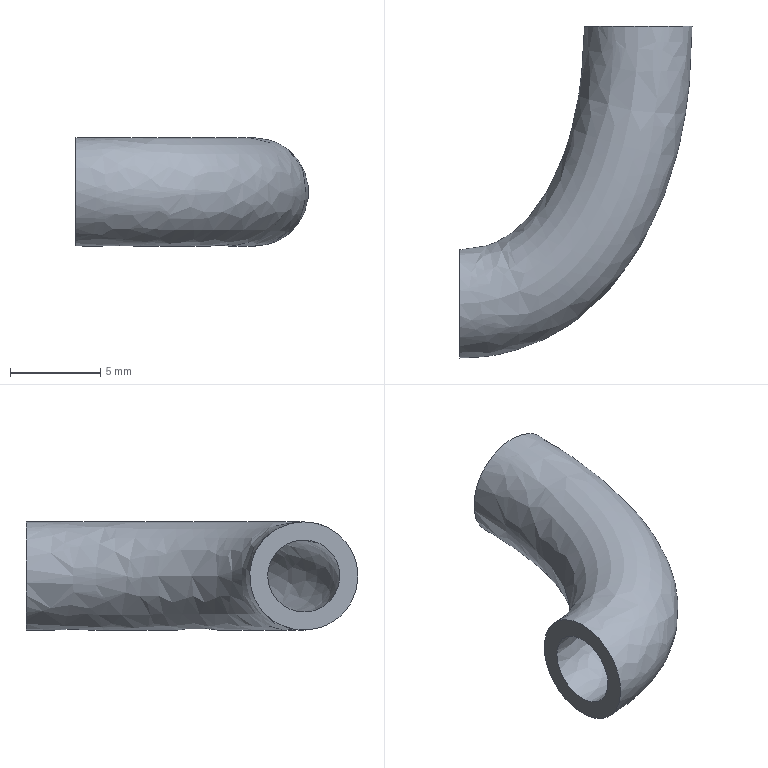Part | NX | features solid 2 | 1 solid | 4 faces | box 12.935 x 18.394 x 6 mm | volume 319.241 mm3 | plane 2 | spline 2